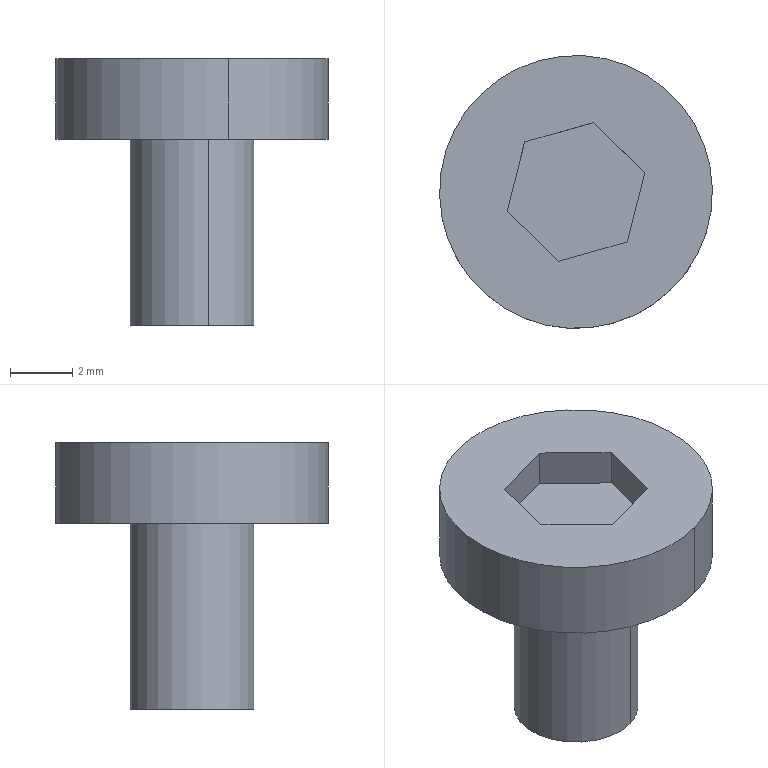Part | NX | features BREP 1 | 1 solid | 14 faces | box 8.8 x 8.8 x 8.6 mm | volume 216.906 mm3 | plane 10 | cylinder 4 | commonest cylinder face diameters 4 x2 8.8 x2
STEP:
#1=CARTESIAN_POINT('',(-11.459,167.35,8.));
#2=VERTEX_POINT('',#1);
#3=CARTESIAN_POINT('',(-12.541,171.2,8.));
#4=VERTEX_POINT('',#3);
#5=CARTESIAN_POINT('',(-12.,169.275,8.));
#6=DIRECTION('',(0.,0.,-1.));
#7=DIRECTION('',(0.2704,-0.9627,0.));
#8=AXIS2_PLACEMENT_3D('',#5,#6,#7);
#9=CIRCLE('',#8,2.);
#10=EDGE_CURVE('',#2,#4,#9,.T.);
#11=ORIENTED_EDGE('',*,*,#10,.F.);
#12=CARTESIAN_POINT('',(-11.459,167.35,14.));
#13=VERTEX_POINT('',#12);
#14=CARTESIAN_POINT('',(-11.459,167.35,8.));
#15=DIRECTION('',(0.,0.,1.));
#16=VECTOR('',#15,1000.);
#17=LINE('',#14,#16);
#18=EDGE_CURVE('',#2,#13,#17,.T.);
#19=ORIENTED_EDGE('',*,*,#18,.T.);
#20=CARTESIAN_POINT('',(-12.541,171.2,14.));
#21=VERTEX_POINT('',#20);
#22=CARTESIAN_POINT('',(-12.,169.275,14.));
#23=DIRECTION('',(0.,0.,-1.));
#24=DIRECTION('',(0.2704,-0.9627,0.));
#25=AXIS2_PLACEMENT_3D('',#22,#23,#24);
#26=CIRCLE('',#25,2.);
#27=EDGE_CURVE('',#13,#21,#26,.T.);
#28=ORIENTED_EDGE('',*,*,#27,.T.);
#29=CARTESIAN_POINT('',(-12.541,171.2,8.));
#30=DIRECTION('',(0.,0.,-1.));
#31=VECTOR('',#30,1000.);
#32=LINE('',#29,#31);
#33=EDGE_CURVE('',#21,#4,#32,.T.);
#34=ORIENTED_EDGE('',*,*,#33,.T.);
#35=EDGE_LOOP('',(#11,#19,#28,#34));
#36=FACE_BOUND('',#35,.T.);
#37=CARTESIAN_POINT('',(-12.,169.275,8.));
#38=DIRECTION('',(0.,0.,1.));
#39=DIRECTION('',(0.2704,-0.9627,0.));
#40=AXIS2_PLACEMENT_3D('',#37,#38,#39);
#41=CYLINDRICAL_SURFACE('',#40,2.);
#42=ADVANCED_FACE('',(#36),#41,.T.);
#43=CARTESIAN_POINT('',(-10.81,165.039,14.));
#44=VERTEX_POINT('',#43);
#45=CARTESIAN_POINT('',(-13.19,173.511,14.));
#46=VERTEX_POINT('',#45);
#47=CARTESIAN_POINT('',(-12.,169.275,14.));
#48=DIRECTION('',(0.,0.,-1.));
#49=DIRECTION('',(0.2704,-0.9627,0.));
#50=AXIS2_PLACEMENT_3D('',#47,#48,#49);
#51=CIRCLE('',#50,4.4);
#52=EDGE_CURVE('',#44,#46,#51,.T.);
#53=ORIENTED_EDGE('',*,*,#52,.F.);
#54=CARTESIAN_POINT('',(-10.81,165.039,16.6));
#55=VERTEX_POINT('',#54);
#56=CARTESIAN_POINT('',(-10.81,165.039,14.));
#57=DIRECTION('',(0.,0.,-1.));
#58=VECTOR('',#57,1000.);
#59=LINE('',#56,#58);
#60=EDGE_CURVE('',#55,#44,#59,.T.);
#61=ORIENTED_EDGE('',*,*,#60,.F.);
#62=CARTESIAN_POINT('',(-13.19,173.511,16.6));
#63=VERTEX_POINT('',#62);
#64=CARTESIAN_POINT('',(-12.,169.275,16.6));
#65=DIRECTION('',(0.,0.,-1.));
#66=DIRECTION('',(0.2704,-0.9627,0.));
#67=AXIS2_PLACEMENT_3D('',#64,#65,#66);
#68=CIRCLE('',#67,4.4);
#69=EDGE_CURVE('',#55,#63,#68,.T.);
#70=ORIENTED_EDGE('',*,*,#69,.T.);
#71=CARTESIAN_POINT('',(-13.19,173.511,14.));
#72=DIRECTION('',(0.,0.,1.));
#73=VECTOR('',#72,1000.);
#74=LINE('',#71,#73);
#75=EDGE_CURVE('',#46,#63,#74,.T.);
#76=ORIENTED_EDGE('',*,*,#75,.F.);
#77=EDGE_LOOP('',(#53,#61,#70,#76));
#78=FACE_BOUND('',#77,.T.);
#79=CARTESIAN_POINT('',(-12.,169.275,14.));
#80=DIRECTION('',(0.,0.,1.));
#81=DIRECTION('',(0.2704,-0.9627,0.));
#82=AXIS2_PLACEMENT_3D('',#79,#80,#81);
#83=CYLINDRICAL_SURFACE('',#82,4.4);
#84=ADVANCED_FACE('',(#78),#83,.T.);
#85=CARTESIAN_POINT('',(-12.,169.275,16.6));
#86=DIRECTION('',(0.,0.,-1.));
#87=DIRECTION('',(0.2704,-0.9627,0.));
#88=AXIS2_PLACEMENT_3D('',#85,#86,#87);
#89=CIRCLE('',#88,4.4);
#90=EDGE_CURVE('',#63,#55,#89,.T.);
#91=ORIENTED_EDGE('',*,*,#90,.F.);
#92=ORIENTED_EDGE('',*,*,#69,.F.);
#93=EDGE_LOOP('',(#91,#92));
#94=FACE_BOUND('',#93,.T.);
#95=CARTESIAN_POINT('',(-10.348,167.662,16.6));
#96=VERTEX_POINT('',#95);
#97=CARTESIAN_POINT('',(-12.571,167.037,16.6));
#98=VERTEX_POINT('',#97);
#99=CARTESIAN_POINT('',(-11.459,167.35,16.6));
#100=DIRECTION('',(-0.9627,-0.2704,0.));
#101=VECTOR('',#100,1000.);
#102=LINE('',#99,#101);
#103=EDGE_CURVE('',#96,#98,#102,.T.);
#104=ORIENTED_EDGE('',*,*,#103,.T.);
#105=CARTESIAN_POINT('',(-14.223,168.651,16.6));
#106=VERTEX_POINT('',#105);
#107=CARTESIAN_POINT('',(-13.397,167.844,16.6));
#108=DIRECTION('',(-0.7155,0.6986,0.));
#109=VECTOR('',#108,1000.);
#110=LINE('',#107,#109);
#111=EDGE_CURVE('',#98,#106,#110,.T.);
#112=ORIENTED_EDGE('',*,*,#111,.T.);
#113=CARTESIAN_POINT('',(-13.652,170.888,16.6));
#114=VERTEX_POINT('',#113);
#115=CARTESIAN_POINT('',(-13.938,169.769,16.6));
#116=DIRECTION('',(0.2472,0.969,0.));
#117=VECTOR('',#116,1000.);
#118=LINE('',#115,#117);
#119=EDGE_CURVE('',#106,#114,#118,.T.);
#120=ORIENTED_EDGE('',*,*,#119,.T.);
#121=CARTESIAN_POINT('',(-11.429,171.513,16.6));
#122=VERTEX_POINT('',#121);
#123=CARTESIAN_POINT('',(-12.541,171.2,16.6));
#124=DIRECTION('',(0.9627,0.2704,0.));
#125=VECTOR('',#124,1000.);
#126=LINE('',#123,#125);
#127=EDGE_CURVE('',#114,#122,#126,.T.);
#128=ORIENTED_EDGE('',*,*,#127,.T.);
#129=CARTESIAN_POINT('',(-9.777,169.899,16.6));
#130=VERTEX_POINT('',#129);
#131=CARTESIAN_POINT('',(-10.603,170.706,16.6));
#132=DIRECTION('',(0.7155,-0.6986,0.));
#133=VECTOR('',#132,1000.);
#134=LINE('',#131,#133);
#135=EDGE_CURVE('',#122,#130,#134,.T.);
#136=ORIENTED_EDGE('',*,*,#135,.T.);
#137=CARTESIAN_POINT('',(-10.062,168.781,16.6));
#138=DIRECTION('',(-0.2472,-0.969,0.));
#139=VECTOR('',#138,1000.);
#140=LINE('',#137,#139);
#141=EDGE_CURVE('',#130,#96,#140,.T.);
#142=ORIENTED_EDGE('',*,*,#141,.T.);
#143=EDGE_LOOP('',(#104,#112,#120,#128,#136,#142));
#144=FACE_BOUND('',#143,.T.);
#145=CARTESIAN_POINT('',(-12.,169.275,16.6));
#146=DIRECTION('',(0.,0.,-1.));
#147=DIRECTION('',(-0.2704,0.9627,0.));
#148=AXIS2_PLACEMENT_3D('',#145,#146,#147);
#149=PLANE('',#148);
#150=ADVANCED_FACE('',(#94,#144),#149,.F.);
#151=CARTESIAN_POINT('',(-12.,169.275,14.));
#152=DIRECTION('',(0.,0.,-1.));
#153=DIRECTION('',(0.2704,-0.9627,0.));
#154=AXIS2_PLACEMENT_3D('',#151,#152,#153);
#155=CIRCLE('',#154,2.);
#156=EDGE_CURVE('',#21,#13,#155,.T.);
#157=ORIENTED_EDGE('',*,*,#156,.F.);
#158=ORIENTED_EDGE('',*,*,#27,.F.);
#159=EDGE_LOOP('',(#157,#158));
#160=FACE_BOUND('',#159,.T.);
#161=CARTESIAN_POINT('',(-12.,169.275,14.));
#162=DIRECTION('',(0.,0.,-1.));
#163=DIRECTION('',(0.2704,-0.9627,0.));
#164=AXIS2_PLACEMENT_3D('',#161,#162,#163);
#165=CIRCLE('',#164,4.4);
#166=EDGE_CURVE('',#46,#44,#165,.T.);
#167=ORIENTED_EDGE('',*,*,#166,.T.);
#168=ORIENTED_EDGE('',*,*,#52,.T.);
#169=EDGE_LOOP('',(#167,#168));
#170=FACE_BOUND('',#169,.T.);
#171=CARTESIAN_POINT('',(-12.,169.275,14.));
#172=DIRECTION('',(0.,0.,-1.));
#173=DIRECTION('',(-0.2704,0.9627,0.));
#174=AXIS2_PLACEMENT_3D('',#171,#172,#173);
#175=PLANE('',#174);
#176=ADVANCED_FACE('',(#160,#170),#175,.T.);
#177=ORIENTED_EDGE('',*,*,#60,.T.);
#178=ORIENTED_EDGE('',*,*,#166,.F.);
#179=ORIENTED_EDGE('',*,*,#75,.T.);
#180=ORIENTED_EDGE('',*,*,#90,.T.);
#181=EDGE_LOOP('',(#177,#178,#179,#180));
#182=FACE_BOUND('',#181,.T.);
#183=CARTESIAN_POINT('',(-12.,169.275,14.));
#184=DIRECTION('',(0.,0.,1.));
#185=DIRECTION('',(0.2704,-0.9627,0.));
#186=AXIS2_PLACEMENT_3D('',#183,#184,#185);
#187=CYLINDRICAL_SURFACE('',#186,4.4);
#188=ADVANCED_FACE('',(#182),#187,.T.);
#189=ORIENTED_EDGE('',*,*,#103,.F.);
#190=CARTESIAN_POINT('',(-10.348,167.662,15.4));
#191=VERTEX_POINT('',#190);
#192=CARTESIAN_POINT('',(-10.348,167.662,15.4));
#193=DIRECTION('',(0.,0.,1.));
#194=VECTOR('',#193,1000.);
#195=LINE('',#192,#194);
#196=EDGE_CURVE('',#191,#96,#195,.T.);
#197=ORIENTED_EDGE('',*,*,#196,.F.);
#198=CARTESIAN_POINT('',(-12.571,167.037,15.4));
#199=VERTEX_POINT('',#198);
#200=CARTESIAN_POINT('',(-11.459,167.35,15.4));
#201=DIRECTION('',(-0.9627,-0.2704,0.));
#202=VECTOR('',#201,1000.);
#203=LINE('',#200,#202);
#204=EDGE_CURVE('',#191,#199,#203,.T.);
#205=ORIENTED_EDGE('',*,*,#204,.T.);
#206=CARTESIAN_POINT('',(-12.571,167.037,15.4));
#207=DIRECTION('',(0.,0.,1.));
#208=VECTOR('',#207,1000.);
#209=LINE('',#206,#208);
#210=EDGE_CURVE('',#199,#98,#209,.T.);
#211=ORIENTED_EDGE('',*,*,#210,.T.);
#212=EDGE_LOOP('',(#189,#197,#205,#211));
#213=FACE_BOUND('',#212,.T.);
#214=CARTESIAN_POINT('',(-11.459,167.35,15.4));
#215=DIRECTION('',(-0.2704,0.9627,0.));
#216=DIRECTION('',(-0.9627,-0.2704,0.));
#217=AXIS2_PLACEMENT_3D('',#214,#215,#216);
#218=PLANE('',#217);
#219=ADVANCED_FACE('',(#213),#218,.T.);
#220=ORIENTED_EDGE('',*,*,#111,.F.);
#221=ORIENTED_EDGE('',*,*,#210,.F.);
#222=CARTESIAN_POINT('',(-14.223,168.651,15.4));
#223=VERTEX_POINT('',#222);
#224=CARTESIAN_POINT('',(-13.397,167.844,15.4));
#225=DIRECTION('',(-0.7155,0.6986,0.));
#226=VECTOR('',#225,1000.);
#227=LINE('',#224,#226);
#228=EDGE_CURVE('',#199,#223,#227,.T.);
#229=ORIENTED_EDGE('',*,*,#228,.T.);
#230=CARTESIAN_POINT('',(-14.223,168.651,15.4));
#231=DIRECTION('',(0.,0.,1.));
#232=VECTOR('',#231,1000.);
#233=LINE('',#230,#232);
#234=EDGE_CURVE('',#223,#106,#233,.T.);
#235=ORIENTED_EDGE('',*,*,#234,.T.);
#236=EDGE_LOOP('',(#220,#221,#229,#235));
#237=FACE_BOUND('',#236,.T.);
#238=CARTESIAN_POINT('',(-13.397,167.844,15.4));
#239=DIRECTION('',(0.6986,0.7155,0.));
#240=DIRECTION('',(-0.7155,0.6986,0.));
#241=AXIS2_PLACEMENT_3D('',#238,#239,#240);
#242=PLANE('',#241);
#243=ADVANCED_FACE('',(#237),#242,.T.);
#244=ORIENTED_EDGE('',*,*,#119,.F.);
#245=ORIENTED_EDGE('',*,*,#234,.F.);
#246=CARTESIAN_POINT('',(-13.652,170.888,15.4));
#247=VERTEX_POINT('',#246);
#248=CARTESIAN_POINT('',(-13.938,169.769,15.4));
#249=DIRECTION('',(0.2472,0.969,0.));
#250=VECTOR('',#249,1000.);
#251=LINE('',#248,#250);
#252=EDGE_CURVE('',#223,#247,#251,.T.);
#253=ORIENTED_EDGE('',*,*,#252,.T.);
#254=CARTESIAN_POINT('',(-13.652,170.888,15.4));
#255=DIRECTION('',(0.,0.,1.));
#256=VECTOR('',#255,1000.);
#257=LINE('',#254,#256);
#258=EDGE_CURVE('',#247,#114,#257,.T.);
#259=ORIENTED_EDGE('',*,*,#258,.T.);
#260=EDGE_LOOP('',(#244,#245,#253,#259));
#261=FACE_BOUND('',#260,.T.);
#262=CARTESIAN_POINT('',(-13.938,169.769,15.4));
#263=DIRECTION('',(0.969,-0.2472,0.));
#264=DIRECTION('',(0.2472,0.969,0.));
#265=AXIS2_PLACEMENT_3D('',#262,#263,#264);
#266=PLANE('',#265);
#267=ADVANCED_FACE('',(#261),#266,.T.);
#268=ORIENTED_EDGE('',*,*,#127,.F.);
#269=ORIENTED_EDGE('',*,*,#258,.F.);
#270=CARTESIAN_POINT('',(-11.429,171.513,15.4));
#271=VERTEX_POINT('',#270);
#272=CARTESIAN_POINT('',(-12.541,171.2,15.4));
#273=DIRECTION('',(0.9627,0.2704,0.));
#274=VECTOR('',#273,1000.);
#275=LINE('',#272,#274);
#276=EDGE_CURVE('',#247,#271,#275,.T.);
#277=ORIENTED_EDGE('',*,*,#276,.T.);
#278=CARTESIAN_POINT('',(-11.429,171.513,15.4));
#279=DIRECTION('',(0.,0.,1.));
#280=VECTOR('',#279,1000.);
#281=LINE('',#278,#280);
#282=EDGE_CURVE('',#271,#122,#281,.T.);
#283=ORIENTED_EDGE('',*,*,#282,.T.);
#284=EDGE_LOOP('',(#268,#269,#277,#283));
#285=FACE_BOUND('',#284,.T.);
#286=CARTESIAN_POINT('',(-12.541,171.2,15.4));
#287=DIRECTION('',(0.2704,-0.9627,0.));
#288=DIRECTION('',(0.9627,0.2704,0.));
#289=AXIS2_PLACEMENT_3D('',#286,#287,#288);
#290=PLANE('',#289);
#291=ADVANCED_FACE('',(#285),#290,.T.);
#292=ORIENTED_EDGE('',*,*,#135,.F.);
#293=ORIENTED_EDGE('',*,*,#282,.F.);
#294=CARTESIAN_POINT('',(-9.777,169.899,15.4));
#295=VERTEX_POINT('',#294);
#296=CARTESIAN_POINT('',(-10.603,170.706,15.4));
#297=DIRECTION('',(0.7155,-0.6986,0.));
#298=VECTOR('',#297,1000.);
#299=LINE('',#296,#298);
#300=EDGE_CURVE('',#271,#295,#299,.T.);
#301=ORIENTED_EDGE('',*,*,#300,.T.);
#302=CARTESIAN_POINT('',(-9.777,169.899,15.4));
#303=DIRECTION('',(0.,0.,1.));
#304=VECTOR('',#303,1000.);
#305=LINE('',#302,#304);
#306=EDGE_CURVE('',#295,#130,#305,.T.);
#307=ORIENTED_EDGE('',*,*,#306,.T.);
#308=EDGE_LOOP('',(#292,#293,#301,#307));
#309=FACE_BOUND('',#308,.T.);
#310=CARTESIAN_POINT('',(-10.603,170.706,15.4));
#311=DIRECTION('',(-0.6986,-0.7155,0.));
#312=DIRECTION('',(0.7155,-0.6986,0.));
#313=AXIS2_PLACEMENT_3D('',#310,#311,#312);
#314=PLANE('',#313);
#315=ADVANCED_FACE('',(#309),#314,.T.);
#316=ORIENTED_EDGE('',*,*,#141,.F.);
#317=ORIENTED_EDGE('',*,*,#306,.F.);
#318=CARTESIAN_POINT('',(-10.062,168.781,15.4));
#319=DIRECTION('',(-0.2472,-0.969,0.));
#320=VECTOR('',#319,1000.);
#321=LINE('',#318,#320);
#322=EDGE_CURVE('',#295,#191,#321,.T.);
#323=ORIENTED_EDGE('',*,*,#322,.T.);
#324=ORIENTED_EDGE('',*,*,#196,.T.);
#325=EDGE_LOOP('',(#316,#317,#323,#324));
#326=FACE_BOUND('',#325,.T.);
#327=CARTESIAN_POINT('',(-10.062,168.781,15.4));
#328=DIRECTION('',(-0.969,0.2472,0.));
#329=DIRECTION('',(-0.2472,-0.969,0.));
#330=AXIS2_PLACEMENT_3D('',#327,#328,#329);
#331=PLANE('',#330);
#332=ADVANCED_FACE('',(#326),#331,.T.);
#333=ORIENTED_EDGE('',*,*,#204,.F.);
#334=ORIENTED_EDGE('',*,*,#322,.F.);
#335=ORIENTED_EDGE('',*,*,#300,.F.);
#336=ORIENTED_EDGE('',*,*,#276,.F.);
#337=ORIENTED_EDGE('',*,*,#252,.F.);
#338=ORIENTED_EDGE('',*,*,#228,.F.);
#339=EDGE_LOOP('',(#333,#334,#335,#336,#337,#338));
#340=FACE_BOUND('',#339,.T.);
#341=CARTESIAN_POINT('',(-12.,169.275,15.4));
#342=DIRECTION('',(0.,0.,-1.));
#343=DIRECTION('',(-0.2704,0.9627,0.));
#344=AXIS2_PLACEMENT_3D('',#341,#342,#343);
#345=PLANE('',#344);
#346=ADVANCED_FACE('',(#340),#345,.F.);
#347=ORIENTED_EDGE('',*,*,#18,.F.);
#348=CARTESIAN_POINT('',(-12.,169.275,8.));
#349=DIRECTION('',(0.,0.,-1.));
#350=DIRECTION('',(0.2704,-0.9627,0.));
#351=AXIS2_PLACEMENT_3D('',#348,#349,#350);
#352=CIRCLE('',#351,2.);
#353=EDGE_CURVE('',#4,#2,#352,.T.);
#354=ORIENTED_EDGE('',*,*,#353,.F.);
#355=ORIENTED_EDGE('',*,*,#33,.F.);
#356=ORIENTED_EDGE('',*,*,#156,.T.);
#357=EDGE_LOOP('',(#347,#354,#355,#356));
#358=FACE_BOUND('',#357,.T.);
#359=CARTESIAN_POINT('',(-12.,169.275,8.));
#360=DIRECTION('',(0.,0.,1.));
#361=DIRECTION('',(0.2704,-0.9627,0.));
#362=AXIS2_PLACEMENT_3D('',#359,#360,#361);
#363=CYLINDRICAL_SURFACE('',#362,2.);
#364=ADVANCED_FACE('',(#358),#363,.T.);
#365=ORIENTED_EDGE('',*,*,#353,.T.);
#366=ORIENTED_EDGE('',*,*,#10,.T.);
#367=EDGE_LOOP('',(#365,#366));
#368=FACE_BOUND('',#367,.T.);
#369=CARTESIAN_POINT('',(-12.,169.275,8.));
#370=DIRECTION('',(0.,0.,-1.));
#371=DIRECTION('',(-0.2704,0.9627,0.));
#372=AXIS2_PLACEMENT_3D('',#369,#370,#371);
#373=PLANE('',#372);
#374=ADVANCED_FACE('',(#368),#373,.T.);
#375=CLOSED_SHELL('',(#42,#84,#150,#176,#188,#219,#243,#267,#291,#315,#332,#346,#364,#374));
#376=MANIFOLD_SOLID_BREP('',#375);
#377=(LENGTH_UNIT()NAMED_UNIT(*)SI_UNIT(.MILLI.,.METRE.));
#378=UNCERTAINTY_MEASURE_WITH_UNIT(LENGTH_MEASURE(0.00001),#377,'','');
#379=(NAMED_UNIT(*)PLANE_ANGLE_UNIT()SI_UNIT($,.RADIAN.));
#380=(NAMED_UNIT(*)SI_UNIT($,.STERADIAN.)SOLID_ANGLE_UNIT());
#381=(GEOMETRIC_REPRESENTATION_CONTEXT(3)GLOBAL_UNCERTAINTY_ASSIGNED_CONTEXT((#378))GLOBAL_UNIT_ASSIGNED_CONTEXT((#377,#379,#380))REPRESENTATION_CONTEXT('',''));
#382=ADVANCED_BREP_SHAPE_REPRESENTATION('',(#376),#381);